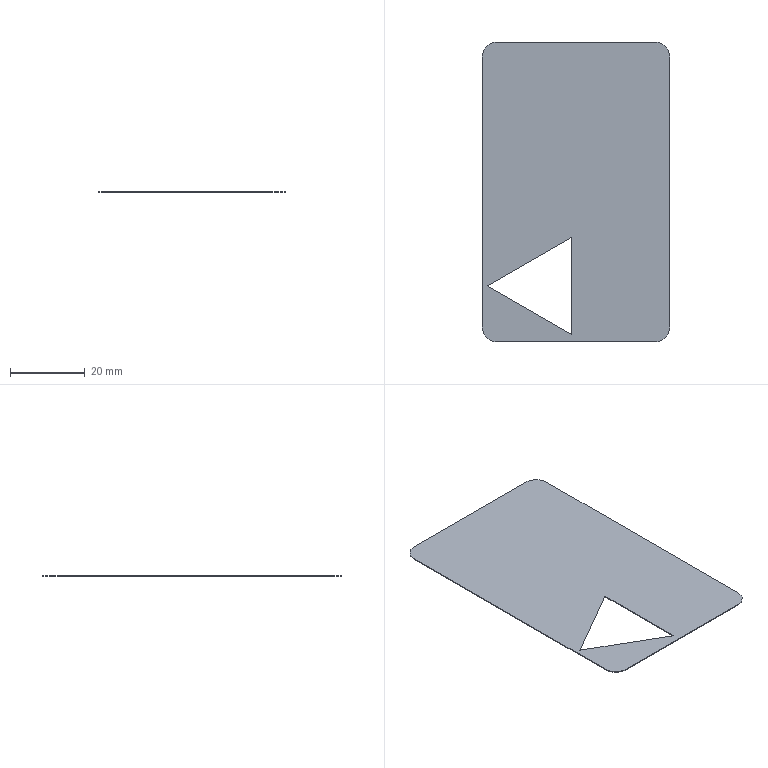Part | SolidWorks | features BaseBody 1 | 1 solid | 13 faces | box 50 x 80 x 0.2 mm | volume 739.101 mm3 | plane 9 | cylinder 4 | commonest cylinder face diameters 8 x4
STEP:
#1=CARTESIAN_POINT('',(204.359,-25.066,330.5));
#2=VERTEX_POINT('',#1);
#3=CARTESIAN_POINT('',(226.8,-38.022,330.5));
#4=VERTEX_POINT('',#3);
#5=CARTESIAN_POINT('',(204.359,-25.066,330.5));
#6=DIRECTION('',(0.866,-0.5,0.));
#7=VECTOR('',#6,1000.);
#8=LINE('',#5,#7);
#9=EDGE_CURVE('',#2,#4,#8,.T.);
#10=ORIENTED_EDGE('',*,*,#9,.T.);
#11=CARTESIAN_POINT('',(226.8,-12.109,330.5));
#12=VERTEX_POINT('',#11);
#13=CARTESIAN_POINT('',(226.8,-38.022,330.5));
#14=DIRECTION('',(0.,1.,0.));
#15=VECTOR('',#14,1000.);
#16=LINE('',#13,#15);
#17=EDGE_CURVE('',#4,#12,#16,.T.);
#18=ORIENTED_EDGE('',*,*,#17,.T.);
#19=CARTESIAN_POINT('',(226.8,-12.109,330.5));
#20=DIRECTION('',(-0.866,-0.5,0.));
#21=VECTOR('',#20,1000.);
#22=LINE('',#19,#21);
#23=EDGE_CURVE('',#12,#2,#22,.T.);
#24=ORIENTED_EDGE('',*,*,#23,.T.);
#25=EDGE_LOOP('',(#10,#18,#24));
#26=FACE_BOUND('',#25,.T.);
#27=CARTESIAN_POINT('',(249.,-40.,330.5));
#28=VERTEX_POINT('',#27);
#29=CARTESIAN_POINT('',(207.,-40.,330.5));
#30=VERTEX_POINT('',#29);
#31=CARTESIAN_POINT('',(249.,-40.,330.5));
#32=DIRECTION('',(-1.,0.,0.));
#33=VECTOR('',#32,1000.);
#34=LINE('',#31,#33);
#35=EDGE_CURVE('',#28,#30,#34,.T.);
#36=ORIENTED_EDGE('',*,*,#35,.T.);
#37=CARTESIAN_POINT('',(203.,-36.,330.5));
#38=VERTEX_POINT('',#37);
#39=CARTESIAN_POINT('',(207.,-36.,330.5));
#40=DIRECTION('',(0.,0.,-1.));
#41=DIRECTION('',(0.,1.,0.));
#42=AXIS2_PLACEMENT_3D('',#39,#40,#41);
#43=CIRCLE('',#42,4.);
#44=EDGE_CURVE('',#30,#38,#43,.T.);
#45=ORIENTED_EDGE('',*,*,#44,.T.);
#46=CARTESIAN_POINT('',(203.,36.,330.5));
#47=VERTEX_POINT('',#46);
#48=CARTESIAN_POINT('',(203.,-36.,330.5));
#49=DIRECTION('',(0.,1.,0.));
#50=VECTOR('',#49,1000.);
#51=LINE('',#48,#50);
#52=EDGE_CURVE('',#38,#47,#51,.T.);
#53=ORIENTED_EDGE('',*,*,#52,.T.);
#54=CARTESIAN_POINT('',(207.,40.,330.5));
#55=VERTEX_POINT('',#54);
#56=CARTESIAN_POINT('',(207.,36.,330.5));
#57=DIRECTION('',(0.,0.,-1.));
#58=DIRECTION('',(0.,1.,0.));
#59=AXIS2_PLACEMENT_3D('',#56,#57,#58);
#60=CIRCLE('',#59,4.);
#61=EDGE_CURVE('',#47,#55,#60,.T.);
#62=ORIENTED_EDGE('',*,*,#61,.T.);
#63=CARTESIAN_POINT('',(249.,40.,330.5));
#64=VERTEX_POINT('',#63);
#65=CARTESIAN_POINT('',(207.,40.,330.5));
#66=DIRECTION('',(1.,0.,0.));
#67=VECTOR('',#66,1000.);
#68=LINE('',#65,#67);
#69=EDGE_CURVE('',#55,#64,#68,.T.);
#70=ORIENTED_EDGE('',*,*,#69,.T.);
#71=CARTESIAN_POINT('',(253.,36.,330.5));
#72=VERTEX_POINT('',#71);
#73=CARTESIAN_POINT('',(249.,36.,330.5));
#74=DIRECTION('',(0.,0.,-1.));
#75=DIRECTION('',(0.,1.,0.));
#76=AXIS2_PLACEMENT_3D('',#73,#74,#75);
#77=CIRCLE('',#76,4.);
#78=EDGE_CURVE('',#64,#72,#77,.T.);
#79=ORIENTED_EDGE('',*,*,#78,.T.);
#80=CARTESIAN_POINT('',(253.,-36.,330.5));
#81=VERTEX_POINT('',#80);
#82=CARTESIAN_POINT('',(253.,36.,330.5));
#83=DIRECTION('',(0.,-1.,0.));
#84=VECTOR('',#83,1000.);
#85=LINE('',#82,#84);
#86=EDGE_CURVE('',#72,#81,#85,.T.);
#87=ORIENTED_EDGE('',*,*,#86,.T.);
#88=CARTESIAN_POINT('',(249.,-36.,330.5));
#89=DIRECTION('',(0.,0.,-1.));
#90=DIRECTION('',(0.,1.,0.));
#91=AXIS2_PLACEMENT_3D('',#88,#89,#90);
#92=CIRCLE('',#91,4.);
#93=EDGE_CURVE('',#81,#28,#92,.T.);
#94=ORIENTED_EDGE('',*,*,#93,.T.);
#95=EDGE_LOOP('',(#36,#45,#53,#62,#70,#79,#87,#94));
#96=FACE_OUTER_BOUND('',#95,.T.);
#97=CARTESIAN_POINT('',(207.,-36.,330.5));
#98=DIRECTION('',(0.,0.,-1.));
#99=DIRECTION('',(0.,-1.,0.));
#100=AXIS2_PLACEMENT_3D('',#97,#98,#99);
#101=PLANE('',#100);
#102=ADVANCED_FACE('',(#26,#96),#101,.T.);
#103=CARTESIAN_POINT('',(204.359,-25.066,330.7));
#104=VERTEX_POINT('',#103);
#105=CARTESIAN_POINT('',(226.8,-38.022,330.7));
#106=VERTEX_POINT('',#105);
#107=CARTESIAN_POINT('',(204.359,-25.066,330.7));
#108=DIRECTION('',(0.866,-0.5,0.));
#109=VECTOR('',#108,1000.);
#110=LINE('',#107,#109);
#111=EDGE_CURVE('',#104,#106,#110,.T.);
#112=ORIENTED_EDGE('',*,*,#111,.F.);
#113=CARTESIAN_POINT('',(226.8,-12.109,330.7));
#114=VERTEX_POINT('',#113);
#115=CARTESIAN_POINT('',(226.8,-12.109,330.7));
#116=DIRECTION('',(-0.866,-0.5,0.));
#117=VECTOR('',#116,1000.);
#118=LINE('',#115,#117);
#119=EDGE_CURVE('',#114,#104,#118,.T.);
#120=ORIENTED_EDGE('',*,*,#119,.F.);
#121=CARTESIAN_POINT('',(226.8,-38.022,330.7));
#122=DIRECTION('',(0.,1.,0.));
#123=VECTOR('',#122,1000.);
#124=LINE('',#121,#123);
#125=EDGE_CURVE('',#106,#114,#124,.T.);
#126=ORIENTED_EDGE('',*,*,#125,.F.);
#127=EDGE_LOOP('',(#112,#120,#126));
#128=FACE_BOUND('',#127,.T.);
#129=CARTESIAN_POINT('',(249.,-40.,330.7));
#130=VERTEX_POINT('',#129);
#131=CARTESIAN_POINT('',(207.,-40.,330.7));
#132=VERTEX_POINT('',#131);
#133=CARTESIAN_POINT('',(249.,-40.,330.7));
#134=DIRECTION('',(-1.,0.,0.));
#135=VECTOR('',#134,1000.);
#136=LINE('',#133,#135);
#137=EDGE_CURVE('',#130,#132,#136,.T.);
#138=ORIENTED_EDGE('',*,*,#137,.F.);
#139=CARTESIAN_POINT('',(253.,-36.,330.7));
#140=VERTEX_POINT('',#139);
#141=CARTESIAN_POINT('',(249.,-36.,330.7));
#142=DIRECTION('',(0.,0.,-1.));
#143=DIRECTION('',(0.,1.,0.));
#144=AXIS2_PLACEMENT_3D('',#141,#142,#143);
#145=CIRCLE('',#144,4.);
#146=EDGE_CURVE('',#140,#130,#145,.T.);
#147=ORIENTED_EDGE('',*,*,#146,.F.);
#148=CARTESIAN_POINT('',(253.,36.,330.7));
#149=VERTEX_POINT('',#148);
#150=CARTESIAN_POINT('',(253.,36.,330.7));
#151=DIRECTION('',(0.,-1.,0.));
#152=VECTOR('',#151,1000.);
#153=LINE('',#150,#152);
#154=EDGE_CURVE('',#149,#140,#153,.T.);
#155=ORIENTED_EDGE('',*,*,#154,.F.);
#156=CARTESIAN_POINT('',(249.,40.,330.7));
#157=VERTEX_POINT('',#156);
#158=CARTESIAN_POINT('',(249.,36.,330.7));
#159=DIRECTION('',(0.,0.,-1.));
#160=DIRECTION('',(0.,1.,0.));
#161=AXIS2_PLACEMENT_3D('',#158,#159,#160);
#162=CIRCLE('',#161,4.);
#163=EDGE_CURVE('',#157,#149,#162,.T.);
#164=ORIENTED_EDGE('',*,*,#163,.F.);
#165=CARTESIAN_POINT('',(207.,40.,330.7));
#166=VERTEX_POINT('',#165);
#167=CARTESIAN_POINT('',(207.,40.,330.7));
#168=DIRECTION('',(1.,0.,0.));
#169=VECTOR('',#168,1000.);
#170=LINE('',#167,#169);
#171=EDGE_CURVE('',#166,#157,#170,.T.);
#172=ORIENTED_EDGE('',*,*,#171,.F.);
#173=CARTESIAN_POINT('',(203.,36.,330.7));
#174=VERTEX_POINT('',#173);
#175=CARTESIAN_POINT('',(207.,36.,330.7));
#176=DIRECTION('',(0.,0.,-1.));
#177=DIRECTION('',(0.,1.,0.));
#178=AXIS2_PLACEMENT_3D('',#175,#176,#177);
#179=CIRCLE('',#178,4.);
#180=EDGE_CURVE('',#174,#166,#179,.T.);
#181=ORIENTED_EDGE('',*,*,#180,.F.);
#182=CARTESIAN_POINT('',(203.,-36.,330.7));
#183=VERTEX_POINT('',#182);
#184=CARTESIAN_POINT('',(203.,-36.,330.7));
#185=DIRECTION('',(0.,1.,0.));
#186=VECTOR('',#185,1000.);
#187=LINE('',#184,#186);
#188=EDGE_CURVE('',#183,#174,#187,.T.);
#189=ORIENTED_EDGE('',*,*,#188,.F.);
#190=CARTESIAN_POINT('',(207.,-36.,330.7));
#191=DIRECTION('',(0.,0.,-1.));
#192=DIRECTION('',(0.,1.,0.));
#193=AXIS2_PLACEMENT_3D('',#190,#191,#192);
#194=CIRCLE('',#193,4.);
#195=EDGE_CURVE('',#132,#183,#194,.T.);
#196=ORIENTED_EDGE('',*,*,#195,.F.);
#197=EDGE_LOOP('',(#138,#147,#155,#164,#172,#181,#189,#196));
#198=FACE_OUTER_BOUND('',#197,.T.);
#199=CARTESIAN_POINT('',(207.,-36.,330.7));
#200=DIRECTION('',(0.,0.,-1.));
#201=DIRECTION('',(0.,-1.,0.));
#202=AXIS2_PLACEMENT_3D('',#199,#200,#201);
#203=PLANE('',#202);
#204=ADVANCED_FACE('',(#128,#198),#203,.F.);
#205=ORIENTED_EDGE('',*,*,#23,.F.);
#206=CARTESIAN_POINT('',(226.8,-12.109,330.7));
#207=DIRECTION('',(0.,0.,-1.));
#208=VECTOR('',#207,1000.);
#209=LINE('',#206,#208);
#210=EDGE_CURVE('',#114,#12,#209,.T.);
#211=ORIENTED_EDGE('',*,*,#210,.F.);
#212=ORIENTED_EDGE('',*,*,#119,.T.);
#213=CARTESIAN_POINT('',(204.359,-25.066,330.7));
#214=DIRECTION('',(0.,0.,-1.));
#215=VECTOR('',#214,1000.);
#216=LINE('',#213,#215);
#217=EDGE_CURVE('',#104,#2,#216,.T.);
#218=ORIENTED_EDGE('',*,*,#217,.T.);
#219=EDGE_LOOP('',(#205,#211,#212,#218));
#220=FACE_OUTER_BOUND('',#219,.T.);
#221=CARTESIAN_POINT('',(226.8,-12.109,330.7));
#222=DIRECTION('',(0.5,-0.866,0.));
#223=DIRECTION('',(0.,0.,-1.));
#224=AXIS2_PLACEMENT_3D('',#221,#222,#223);
#225=PLANE('',#224);
#226=ADVANCED_FACE('',(#220),#225,.T.);
#227=ORIENTED_EDGE('',*,*,#93,.F.);
#228=CARTESIAN_POINT('',(253.,-36.,330.7));
#229=DIRECTION('',(0.,0.,-1.));
#230=VECTOR('',#229,1000.);
#231=LINE('',#228,#230);
#232=EDGE_CURVE('',#140,#81,#231,.T.);
#233=ORIENTED_EDGE('',*,*,#232,.F.);
#234=ORIENTED_EDGE('',*,*,#146,.T.);
#235=CARTESIAN_POINT('',(249.,-40.,330.7));
#236=DIRECTION('',(0.,0.,-1.));
#237=VECTOR('',#236,1000.);
#238=LINE('',#235,#237);
#239=EDGE_CURVE('',#130,#28,#238,.T.);
#240=ORIENTED_EDGE('',*,*,#239,.T.);
#241=EDGE_LOOP('',(#227,#233,#234,#240));
#242=FACE_OUTER_BOUND('',#241,.T.);
#243=CARTESIAN_POINT('',(249.,-36.,330.7));
#244=DIRECTION('',(0.,0.,-1.));
#245=DIRECTION('',(0.,-1.,0.));
#246=AXIS2_PLACEMENT_3D('',#243,#244,#245);
#247=CYLINDRICAL_SURFACE('',#246,4.);
#248=ADVANCED_FACE('',(#242),#247,.T.);
#249=ORIENTED_EDGE('',*,*,#86,.F.);
#250=CARTESIAN_POINT('',(253.,36.,330.7));
#251=DIRECTION('',(0.,0.,-1.));
#252=VECTOR('',#251,1000.);
#253=LINE('',#250,#252);
#254=EDGE_CURVE('',#149,#72,#253,.T.);
#255=ORIENTED_EDGE('',*,*,#254,.F.);
#256=ORIENTED_EDGE('',*,*,#154,.T.);
#257=ORIENTED_EDGE('',*,*,#232,.T.);
#258=EDGE_LOOP('',(#249,#255,#256,#257));
#259=FACE_OUTER_BOUND('',#258,.T.);
#260=CARTESIAN_POINT('',(253.,36.,330.7));
#261=DIRECTION('',(1.,0.,0.));
#262=DIRECTION('',(0.,1.,0.));
#263=AXIS2_PLACEMENT_3D('',#260,#261,#262);
#264=PLANE('',#263);
#265=ADVANCED_FACE('',(#259),#264,.T.);
#266=ORIENTED_EDGE('',*,*,#78,.F.);
#267=CARTESIAN_POINT('',(249.,40.,330.7));
#268=DIRECTION('',(0.,0.,-1.));
#269=VECTOR('',#268,1000.);
#270=LINE('',#267,#269);
#271=EDGE_CURVE('',#157,#64,#270,.T.);
#272=ORIENTED_EDGE('',*,*,#271,.F.);
#273=ORIENTED_EDGE('',*,*,#163,.T.);
#274=ORIENTED_EDGE('',*,*,#254,.T.);
#275=EDGE_LOOP('',(#266,#272,#273,#274));
#276=FACE_OUTER_BOUND('',#275,.T.);
#277=CARTESIAN_POINT('',(249.,36.,330.7));
#278=DIRECTION('',(0.,0.,-1.));
#279=DIRECTION('',(0.,-1.,0.));
#280=AXIS2_PLACEMENT_3D('',#277,#278,#279);
#281=CYLINDRICAL_SURFACE('',#280,4.);
#282=ADVANCED_FACE('',(#276),#281,.T.);
#283=ORIENTED_EDGE('',*,*,#69,.F.);
#284=CARTESIAN_POINT('',(207.,40.,330.7));
#285=DIRECTION('',(0.,0.,-1.));
#286=VECTOR('',#285,1000.);
#287=LINE('',#284,#286);
#288=EDGE_CURVE('',#166,#55,#287,.T.);
#289=ORIENTED_EDGE('',*,*,#288,.F.);
#290=ORIENTED_EDGE('',*,*,#171,.T.);
#291=ORIENTED_EDGE('',*,*,#271,.T.);
#292=EDGE_LOOP('',(#283,#289,#290,#291));
#293=FACE_OUTER_BOUND('',#292,.T.);
#294=CARTESIAN_POINT('',(207.,40.,330.7));
#295=DIRECTION('',(0.,1.,0.));
#296=DIRECTION('',(1.,0.,0.));
#297=AXIS2_PLACEMENT_3D('',#294,#295,#296);
#298=PLANE('',#297);
#299=ADVANCED_FACE('',(#293),#298,.T.);
#300=ORIENTED_EDGE('',*,*,#61,.F.);
#301=CARTESIAN_POINT('',(203.,36.,330.7));
#302=DIRECTION('',(0.,0.,-1.));
#303=VECTOR('',#302,1000.);
#304=LINE('',#301,#303);
#305=EDGE_CURVE('',#174,#47,#304,.T.);
#306=ORIENTED_EDGE('',*,*,#305,.F.);
#307=ORIENTED_EDGE('',*,*,#180,.T.);
#308=ORIENTED_EDGE('',*,*,#288,.T.);
#309=EDGE_LOOP('',(#300,#306,#307,#308));
#310=FACE_OUTER_BOUND('',#309,.T.);
#311=CARTESIAN_POINT('',(207.,36.,330.7));
#312=DIRECTION('',(0.,0.,-1.));
#313=DIRECTION('',(0.,-1.,0.));
#314=AXIS2_PLACEMENT_3D('',#311,#312,#313);
#315=CYLINDRICAL_SURFACE('',#314,4.);
#316=ADVANCED_FACE('',(#310),#315,.T.);
#317=ORIENTED_EDGE('',*,*,#52,.F.);
#318=CARTESIAN_POINT('',(203.,-36.,330.7));
#319=DIRECTION('',(0.,0.,-1.));
#320=VECTOR('',#319,1000.);
#321=LINE('',#318,#320);
#322=EDGE_CURVE('',#183,#38,#321,.T.);
#323=ORIENTED_EDGE('',*,*,#322,.F.);
#324=ORIENTED_EDGE('',*,*,#188,.T.);
#325=ORIENTED_EDGE('',*,*,#305,.T.);
#326=EDGE_LOOP('',(#317,#323,#324,#325));
#327=FACE_OUTER_BOUND('',#326,.T.);
#328=CARTESIAN_POINT('',(203.,-36.,330.7));
#329=DIRECTION('',(-1.,0.,0.));
#330=DIRECTION('',(0.,0.,1.));
#331=AXIS2_PLACEMENT_3D('',#328,#329,#330);
#332=PLANE('',#331);
#333=ADVANCED_FACE('',(#327),#332,.T.);
#334=ORIENTED_EDGE('',*,*,#44,.F.);
#335=CARTESIAN_POINT('',(207.,-40.,330.7));
#336=DIRECTION('',(0.,0.,-1.));
#337=VECTOR('',#336,1000.);
#338=LINE('',#335,#337);
#339=EDGE_CURVE('',#132,#30,#338,.T.);
#340=ORIENTED_EDGE('',*,*,#339,.F.);
#341=ORIENTED_EDGE('',*,*,#195,.T.);
#342=ORIENTED_EDGE('',*,*,#322,.T.);
#343=EDGE_LOOP('',(#334,#340,#341,#342));
#344=FACE_OUTER_BOUND('',#343,.T.);
#345=CARTESIAN_POINT('',(207.,-36.,330.7));
#346=DIRECTION('',(0.,0.,-1.));
#347=DIRECTION('',(0.,-1.,0.));
#348=AXIS2_PLACEMENT_3D('',#345,#346,#347);
#349=CYLINDRICAL_SURFACE('',#348,4.);
#350=ADVANCED_FACE('',(#344),#349,.T.);
#351=ORIENTED_EDGE('',*,*,#35,.F.);
#352=ORIENTED_EDGE('',*,*,#239,.F.);
#353=ORIENTED_EDGE('',*,*,#137,.T.);
#354=ORIENTED_EDGE('',*,*,#339,.T.);
#355=EDGE_LOOP('',(#351,#352,#353,#354));
#356=FACE_OUTER_BOUND('',#355,.T.);
#357=CARTESIAN_POINT('',(249.,-40.,330.7));
#358=DIRECTION('',(0.,-1.,0.));
#359=DIRECTION('',(-1.,0.,0.));
#360=AXIS2_PLACEMENT_3D('',#357,#358,#359);
#361=PLANE('',#360);
#362=ADVANCED_FACE('',(#356),#361,.T.);
#363=ORIENTED_EDGE('',*,*,#17,.F.);
#364=CARTESIAN_POINT('',(226.8,-38.022,330.7));
#365=DIRECTION('',(0.,0.,-1.));
#366=VECTOR('',#365,1000.);
#367=LINE('',#364,#366);
#368=EDGE_CURVE('',#106,#4,#367,.T.);
#369=ORIENTED_EDGE('',*,*,#368,.F.);
#370=ORIENTED_EDGE('',*,*,#125,.T.);
#371=ORIENTED_EDGE('',*,*,#210,.T.);
#372=EDGE_LOOP('',(#363,#369,#370,#371));
#373=FACE_OUTER_BOUND('',#372,.T.);
#374=CARTESIAN_POINT('',(226.8,-38.022,330.7));
#375=DIRECTION('',(-1.,0.,0.));
#376=DIRECTION('',(0.,0.,1.));
#377=AXIS2_PLACEMENT_3D('',#374,#375,#376);
#378=PLANE('',#377);
#379=ADVANCED_FACE('',(#373),#378,.T.);
#380=ORIENTED_EDGE('',*,*,#9,.F.);
#381=ORIENTED_EDGE('',*,*,#217,.F.);
#382=ORIENTED_EDGE('',*,*,#111,.T.);
#383=ORIENTED_EDGE('',*,*,#368,.T.);
#384=EDGE_LOOP('',(#380,#381,#382,#383));
#385=FACE_OUTER_BOUND('',#384,.T.);
#386=CARTESIAN_POINT('',(204.359,-25.066,330.7));
#387=DIRECTION('',(0.5,0.866,0.));
#388=DIRECTION('',(0.,0.,-1.));
#389=AXIS2_PLACEMENT_3D('',#386,#387,#388);
#390=PLANE('',#389);
#391=ADVANCED_FACE('',(#385),#390,.T.);
#392=CLOSED_SHELL('',(#102,#204,#226,#248,#265,#282,#299,#316,#333,#350,#362,#379,#391));
#393=MANIFOLD_SOLID_BREP('',#392);
#394=CARTESIAN_POINT('',(0.,0.,0.));
#395=DIRECTION('',(0.,0.,1.));
#396=DIRECTION('',(1.,0.,0.));
#397=AXIS2_PLACEMENT_3D('',#394,#395,#396);
#398=(LENGTH_UNIT()NAMED_UNIT(*)SI_UNIT(.MILLI.,.METRE.));
#399=UNCERTAINTY_MEASURE_WITH_UNIT(LENGTH_MEASURE(0.00001),#398,'','');
#400=(NAMED_UNIT(*)PLANE_ANGLE_UNIT()SI_UNIT($,.RADIAN.));
#401=(NAMED_UNIT(*)SI_UNIT($,.STERADIAN.)SOLID_ANGLE_UNIT());
#402=(GEOMETRIC_REPRESENTATION_CONTEXT(3)GLOBAL_UNCERTAINTY_ASSIGNED_CONTEXT((#399))GLOBAL_UNIT_ASSIGNED_CONTEXT((#398,#400,#401))REPRESENTATION_CONTEXT('',''));
#403=ADVANCED_BREP_SHAPE_REPRESENTATION('',(#393,#397),#402);